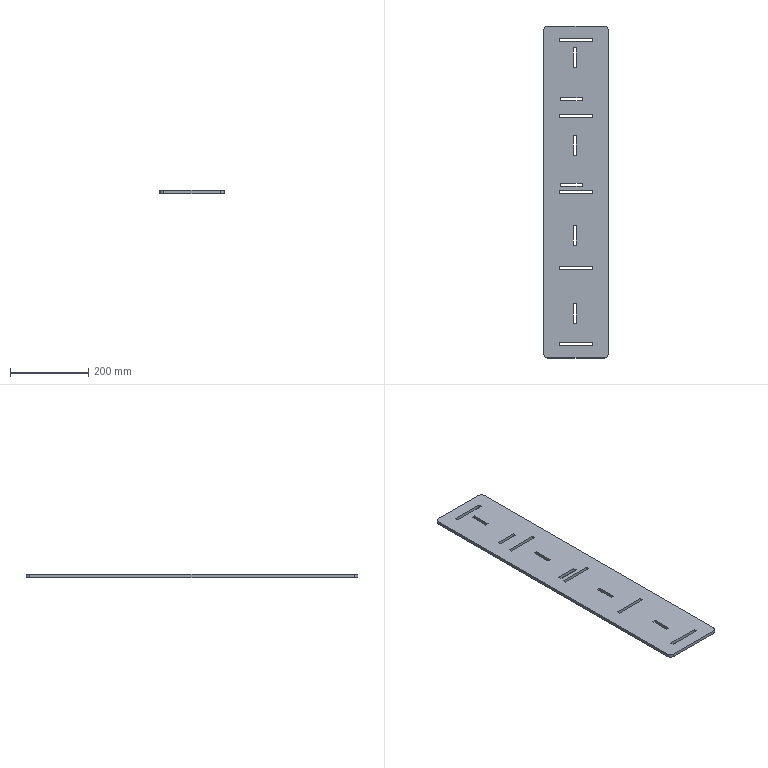Part | SolidWorks | features FlatPattern 1, SMBaseFlange 1, SheetMetal 1 | 1 solid | 54 faces | box 165 x 850 x 8 mm | volume 1074273 mm3 | plane 50 | cylinder 4 | commonest cylinder face diameters 20 x4